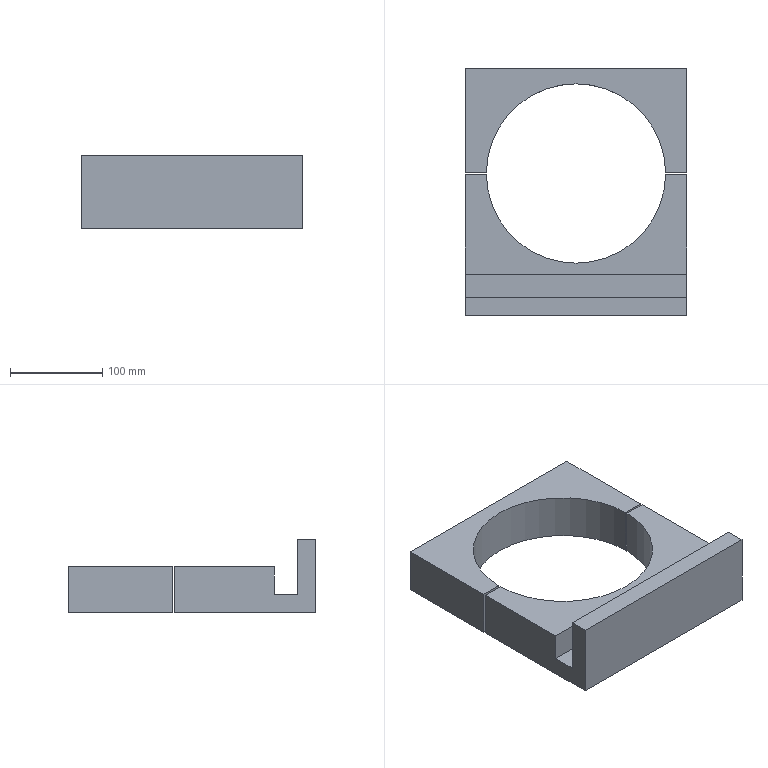Part | STEP file | beam expander fixing.step.STEP-247.STEP | 2 solids | 20 faces | box 240 x 268 x 80 mm | volume 1697437 mm3 | plane 18 | cylinder 2 | commonest cylinder face diameters 194 x2
STEP:
#1=CARTESIAN_POINT('',(96.995,78.,50.));
#2=VERTEX_POINT('',#1);
#3=CARTESIAN_POINT('',(96.995,78.,0.));
#4=VERTEX_POINT('',#3);
#5=CARTESIAN_POINT('',(96.995,78.,50.));
#6=DIRECTION('',(0.,0.,-1.));
#7=VECTOR('',#6,1000.);
#8=LINE('',#5,#7);
#9=EDGE_CURVE('',#2,#4,#8,.T.);
#10=ORIENTED_EDGE('',*,*,#9,.T.);
#11=CARTESIAN_POINT('',(120.,78.,0.));
#12=VERTEX_POINT('',#11);
#13=CARTESIAN_POINT('',(0.,78.,0.));
#14=DIRECTION('',(-1.,0.,0.));
#15=VECTOR('',#14,1000.);
#16=LINE('',#13,#15);
#17=EDGE_CURVE('',#12,#4,#16,.T.);
#18=ORIENTED_EDGE('',*,*,#17,.F.);
#19=CARTESIAN_POINT('',(120.,78.,50.));
#20=VERTEX_POINT('',#19);
#21=CARTESIAN_POINT('',(120.,78.,50.));
#22=DIRECTION('',(0.,0.,1.));
#23=VECTOR('',#22,1000.);
#24=LINE('',#21,#23);
#25=EDGE_CURVE('',#12,#20,#24,.T.);
#26=ORIENTED_EDGE('',*,*,#25,.T.);
#27=CARTESIAN_POINT('',(-163.686,78.,50.));
#28=DIRECTION('',(-1.,0.,0.));
#29=VECTOR('',#28,1000.);
#30=LINE('',#27,#29);
#31=EDGE_CURVE('',#20,#2,#30,.T.);
#32=ORIENTED_EDGE('',*,*,#31,.T.);
#33=EDGE_LOOP('',(#10,#18,#26,#32));
#34=FACE_OUTER_BOUND('',#33,.T.);
#35=CARTESIAN_POINT('',(-163.686,78.,0.));
#36=DIRECTION('',(0.,1.,0.));
#37=DIRECTION('',(1.,0.,0.));
#38=AXIS2_PLACEMENT_3D('',#35,#36,#37);
#39=PLANE('',#38);
#40=ADVANCED_FACE('',(#34),#39,.F.);
#41=CARTESIAN_POINT('',(-96.995,78.,0.));
#42=VERTEX_POINT('',#41);
#43=CARTESIAN_POINT('',(-96.995,78.,50.));
#44=VERTEX_POINT('',#43);
#45=CARTESIAN_POINT('',(-96.995,78.,50.));
#46=DIRECTION('',(0.,0.,1.));
#47=VECTOR('',#46,1000.);
#48=LINE('',#45,#47);
#49=EDGE_CURVE('',#42,#44,#48,.T.);
#50=ORIENTED_EDGE('',*,*,#49,.T.);
#51=CARTESIAN_POINT('',(-120.,78.,50.));
#52=VERTEX_POINT('',#51);
#53=CARTESIAN_POINT('',(-163.686,78.,50.));
#54=DIRECTION('',(-1.,0.,0.));
#55=VECTOR('',#54,1000.);
#56=LINE('',#53,#55);
#57=EDGE_CURVE('',#44,#52,#56,.T.);
#58=ORIENTED_EDGE('',*,*,#57,.T.);
#59=CARTESIAN_POINT('',(-120.,78.,0.));
#60=VERTEX_POINT('',#59);
#61=CARTESIAN_POINT('',(-120.,78.,50.));
#62=DIRECTION('',(0.,0.,1.));
#63=VECTOR('',#62,1000.);
#64=LINE('',#61,#63);
#65=EDGE_CURVE('',#60,#52,#64,.T.);
#66=ORIENTED_EDGE('',*,*,#65,.F.);
#67=CARTESIAN_POINT('',(0.,78.,0.));
#68=DIRECTION('',(-1.,0.,0.));
#69=VECTOR('',#68,1000.);
#70=LINE('',#67,#69);
#71=EDGE_CURVE('',#42,#60,#70,.T.);
#72=ORIENTED_EDGE('',*,*,#71,.F.);
#73=EDGE_LOOP('',(#50,#58,#66,#72));
#74=FACE_OUTER_BOUND('',#73,.T.);
#75=CARTESIAN_POINT('',(-163.686,78.,0.));
#76=DIRECTION('',(0.,1.,0.));
#77=DIRECTION('',(1.,0.,0.));
#78=AXIS2_PLACEMENT_3D('',#75,#76,#77);
#79=PLANE('',#78);
#80=ADVANCED_FACE('',(#74),#79,.F.);
#81=ORIENTED_EDGE('',*,*,#9,.F.);
#82=CARTESIAN_POINT('',(0.,77.,50.));
#83=DIRECTION('',(0.,0.,1.));
#84=DIRECTION('',(1.,0.,0.));
#85=AXIS2_PLACEMENT_3D('',#82,#83,#84);
#86=CIRCLE('',#85,97.);
#87=EDGE_CURVE('',#2,#44,#86,.T.);
#88=ORIENTED_EDGE('',*,*,#87,.T.);
#89=ORIENTED_EDGE('',*,*,#49,.F.);
#90=CARTESIAN_POINT('',(0.,77.,0.));
#91=DIRECTION('',(0.,0.,1.));
#92=DIRECTION('',(1.,0.,0.));
#93=AXIS2_PLACEMENT_3D('',#90,#91,#92);
#94=CIRCLE('',#93,97.);
#95=EDGE_CURVE('',#4,#42,#94,.T.);
#96=ORIENTED_EDGE('',*,*,#95,.F.);
#97=EDGE_LOOP('',(#81,#88,#89,#96));
#98=FACE_OUTER_BOUND('',#97,.T.);
#99=CARTESIAN_POINT('',(0.,77.,50.));
#100=DIRECTION('',(0.,0.,-1.));
#101=DIRECTION('',(-1.,0.,0.));
#102=AXIS2_PLACEMENT_3D('',#99,#100,#101);
#103=CYLINDRICAL_SURFACE('',#102,97.);
#104=ADVANCED_FACE('',(#98),#103,.F.);
#105=CARTESIAN_POINT('',(-120.,191.,0.));
#106=VERTEX_POINT('',#105);
#107=CARTESIAN_POINT('',(-120.,0.,0.));
#108=DIRECTION('',(0.,-1.,0.));
#109=VECTOR('',#108,1000.);
#110=LINE('',#107,#109);
#111=EDGE_CURVE('',#106,#60,#110,.T.);
#112=ORIENTED_EDGE('',*,*,#111,.T.);
#113=ORIENTED_EDGE('',*,*,#65,.T.);
#114=CARTESIAN_POINT('',(-120.,191.,50.));
#115=VERTEX_POINT('',#114);
#116=CARTESIAN_POINT('',(-120.,0.,50.));
#117=DIRECTION('',(0.,-1.,0.));
#118=VECTOR('',#117,1000.);
#119=LINE('',#116,#118);
#120=EDGE_CURVE('',#115,#52,#119,.T.);
#121=ORIENTED_EDGE('',*,*,#120,.F.);
#122=CARTESIAN_POINT('',(-120.,191.,0.));
#123=DIRECTION('',(0.,0.,1.));
#124=VECTOR('',#123,1000.);
#125=LINE('',#122,#124);
#126=EDGE_CURVE('',#106,#115,#125,.T.);
#127=ORIENTED_EDGE('',*,*,#126,.F.);
#128=EDGE_LOOP('',(#112,#113,#121,#127));
#129=FACE_OUTER_BOUND('',#128,.T.);
#130=CARTESIAN_POINT('',(-120.,0.,50.));
#131=DIRECTION('',(1.,0.,0.));
#132=DIRECTION('',(0.,1.,0.));
#133=AXIS2_PLACEMENT_3D('',#130,#131,#132);
#134=PLANE('',#133);
#135=ADVANCED_FACE('',(#129),#134,.F.);
#136=ORIENTED_EDGE('',*,*,#25,.F.);
#137=CARTESIAN_POINT('',(120.,191.,0.));
#138=VERTEX_POINT('',#137);
#139=CARTESIAN_POINT('',(120.,0.,0.));
#140=DIRECTION('',(0.,-1.,0.));
#141=VECTOR('',#140,1000.);
#142=LINE('',#139,#141);
#143=EDGE_CURVE('',#138,#12,#142,.T.);
#144=ORIENTED_EDGE('',*,*,#143,.F.);
#145=CARTESIAN_POINT('',(120.,191.,50.));
#146=VERTEX_POINT('',#145);
#147=CARTESIAN_POINT('',(120.,191.,0.));
#148=DIRECTION('',(0.,0.,1.));
#149=VECTOR('',#148,1000.);
#150=LINE('',#147,#149);
#151=EDGE_CURVE('',#138,#146,#150,.T.);
#152=ORIENTED_EDGE('',*,*,#151,.T.);
#153=CARTESIAN_POINT('',(120.,0.,50.));
#154=DIRECTION('',(0.,-1.,0.));
#155=VECTOR('',#154,1000.);
#156=LINE('',#153,#155);
#157=EDGE_CURVE('',#146,#20,#156,.T.);
#158=ORIENTED_EDGE('',*,*,#157,.T.);
#159=EDGE_LOOP('',(#136,#144,#152,#158));
#160=FACE_OUTER_BOUND('',#159,.T.);
#161=CARTESIAN_POINT('',(120.,0.,50.));
#162=DIRECTION('',(1.,0.,0.));
#163=DIRECTION('',(0.,1.,0.));
#164=AXIS2_PLACEMENT_3D('',#161,#162,#163);
#165=PLANE('',#164);
#166=ADVANCED_FACE('',(#160),#165,.T.);
#167=ORIENTED_EDGE('',*,*,#143,.T.);
#168=ORIENTED_EDGE('',*,*,#17,.T.);
#169=ORIENTED_EDGE('',*,*,#95,.T.);
#170=ORIENTED_EDGE('',*,*,#71,.T.);
#171=ORIENTED_EDGE('',*,*,#111,.F.);
#172=CARTESIAN_POINT('',(-120.,191.,0.));
#173=DIRECTION('',(1.,0.,0.));
#174=VECTOR('',#173,1000.);
#175=LINE('',#172,#174);
#176=EDGE_CURVE('',#106,#138,#175,.T.);
#177=ORIENTED_EDGE('',*,*,#176,.T.);
#178=EDGE_LOOP('',(#167,#168,#169,#170,#171,#177));
#179=FACE_OUTER_BOUND('',#178,.T.);
#180=CARTESIAN_POINT('',(0.,0.,0.));
#181=DIRECTION('',(0.,0.,1.));
#182=DIRECTION('',(1.,0.,0.));
#183=AXIS2_PLACEMENT_3D('',#180,#181,#182);
#184=PLANE('',#183);
#185=ADVANCED_FACE('',(#179),#184,.F.);
#186=ORIENTED_EDGE('',*,*,#31,.F.);
#187=ORIENTED_EDGE('',*,*,#157,.F.);
#188=CARTESIAN_POINT('',(-120.,191.,50.));
#189=DIRECTION('',(1.,0.,0.));
#190=VECTOR('',#189,1000.);
#191=LINE('',#188,#190);
#192=EDGE_CURVE('',#115,#146,#191,.T.);
#193=ORIENTED_EDGE('',*,*,#192,.F.);
#194=ORIENTED_EDGE('',*,*,#120,.T.);
#195=ORIENTED_EDGE('',*,*,#57,.F.);
#196=ORIENTED_EDGE('',*,*,#87,.F.);
#197=EDGE_LOOP('',(#186,#187,#193,#194,#195,#196));
#198=FACE_OUTER_BOUND('',#197,.T.);
#199=CARTESIAN_POINT('',(0.,0.,50.));
#200=DIRECTION('',(0.,0.,1.));
#201=DIRECTION('',(1.,0.,0.));
#202=AXIS2_PLACEMENT_3D('',#199,#200,#201);
#203=PLANE('',#202);
#204=ADVANCED_FACE('',(#198),#203,.T.);
#205=ORIENTED_EDGE('',*,*,#192,.T.);
#206=ORIENTED_EDGE('',*,*,#151,.F.);
#207=ORIENTED_EDGE('',*,*,#176,.F.);
#208=ORIENTED_EDGE('',*,*,#126,.T.);
#209=EDGE_LOOP('',(#205,#206,#207,#208));
#210=FACE_OUTER_BOUND('',#209,.T.);
#211=CARTESIAN_POINT('',(-120.,191.,0.));
#212=DIRECTION('',(0.,-1.,0.));
#213=DIRECTION('',(0.,0.,-1.));
#214=AXIS2_PLACEMENT_3D('',#211,#212,#213);
#215=PLANE('',#214);
#216=ADVANCED_FACE('',(#210),#215,.F.);
#217=CLOSED_SHELL('',(#40,#80,#104,#135,#166,#185,#204,#216));
#218=MANIFOLD_SOLID_BREP('',#217);
#219=CARTESIAN_POINT('',(120.,-57.,20.));
#220=VERTEX_POINT('',#219);
#221=CARTESIAN_POINT('',(120.,-32.,20.));
#222=VERTEX_POINT('',#221);
#223=CARTESIAN_POINT('',(120.,-57.,20.));
#224=DIRECTION('',(0.,1.,0.));
#225=VECTOR('',#224,1000.);
#226=LINE('',#223,#225);
#227=EDGE_CURVE('',#220,#222,#226,.T.);
#228=ORIENTED_EDGE('',*,*,#227,.T.);
#229=CARTESIAN_POINT('',(-120.,-32.,20.));
#230=VERTEX_POINT('',#229);
#231=CARTESIAN_POINT('',(120.,-32.,20.));
#232=DIRECTION('',(-1.,0.,0.));
#233=VECTOR('',#232,1000.);
#234=LINE('',#231,#233);
#235=EDGE_CURVE('',#222,#230,#234,.T.);
#236=ORIENTED_EDGE('',*,*,#235,.T.);
#237=CARTESIAN_POINT('',(-120.,-57.,20.));
#238=VERTEX_POINT('',#237);
#239=CARTESIAN_POINT('',(-120.,-57.,20.));
#240=DIRECTION('',(0.,-1.,0.));
#241=VECTOR('',#240,1000.);
#242=LINE('',#239,#241);
#243=EDGE_CURVE('',#230,#238,#242,.T.);
#244=ORIENTED_EDGE('',*,*,#243,.T.);
#245=CARTESIAN_POINT('',(120.,-57.,20.));
#246=DIRECTION('',(1.,0.,0.));
#247=VECTOR('',#246,1000.);
#248=LINE('',#245,#247);
#249=EDGE_CURVE('',#238,#220,#248,.T.);
#250=ORIENTED_EDGE('',*,*,#249,.T.);
#251=EDGE_LOOP('',(#228,#236,#244,#250));
#252=FACE_OUTER_BOUND('',#251,.T.);
#253=CARTESIAN_POINT('',(0.,0.,20.));
#254=DIRECTION('',(0.,0.,1.));
#255=DIRECTION('',(1.,0.,0.));
#256=AXIS2_PLACEMENT_3D('',#253,#254,#255);
#257=PLANE('',#256);
#258=ADVANCED_FACE('',(#252),#257,.T.);
#259=CARTESIAN_POINT('',(120.,-32.,50.));
#260=VERTEX_POINT('',#259);
#261=CARTESIAN_POINT('',(-120.,-32.,50.));
#262=VERTEX_POINT('',#261);
#263=CARTESIAN_POINT('',(120.,-32.,50.));
#264=DIRECTION('',(-1.,0.,0.));
#265=VECTOR('',#264,1000.);
#266=LINE('',#263,#265);
#267=EDGE_CURVE('',#260,#262,#266,.T.);
#268=ORIENTED_EDGE('',*,*,#267,.T.);
#269=CARTESIAN_POINT('',(-120.,-32.,20.));
#270=DIRECTION('',(0.,0.,1.));
#271=VECTOR('',#270,1000.);
#272=LINE('',#269,#271);
#273=EDGE_CURVE('',#230,#262,#272,.T.);
#274=ORIENTED_EDGE('',*,*,#273,.F.);
#275=ORIENTED_EDGE('',*,*,#235,.F.);
#276=CARTESIAN_POINT('',(120.,-32.,20.));
#277=DIRECTION('',(0.,0.,1.));
#278=VECTOR('',#277,1000.);
#279=LINE('',#276,#278);
#280=EDGE_CURVE('',#222,#260,#279,.T.);
#281=ORIENTED_EDGE('',*,*,#280,.T.);
#282=EDGE_LOOP('',(#268,#274,#275,#281));
#283=FACE_OUTER_BOUND('',#282,.T.);
#284=CARTESIAN_POINT('',(120.,-32.,20.));
#285=DIRECTION('',(0.,1.,0.));
#286=DIRECTION('',(1.,0.,0.));
#287=AXIS2_PLACEMENT_3D('',#284,#285,#286);
#288=PLANE('',#287);
#289=ADVANCED_FACE('',(#283),#288,.F.);
#290=CARTESIAN_POINT('',(-120.,-57.,80.));
#291=VERTEX_POINT('',#290);
#292=CARTESIAN_POINT('',(-120.,-77.,80.));
#293=VERTEX_POINT('',#292);
#294=CARTESIAN_POINT('',(-120.,-77.,80.));
#295=DIRECTION('',(0.,-1.,0.));
#296=VECTOR('',#295,1000.);
#297=LINE('',#294,#296);
#298=EDGE_CURVE('',#291,#293,#297,.T.);
#299=ORIENTED_EDGE('',*,*,#298,.T.);
#300=CARTESIAN_POINT('',(120.,-77.,80.));
#301=VERTEX_POINT('',#300);
#302=CARTESIAN_POINT('',(-120.,-77.,80.));
#303=DIRECTION('',(1.,0.,0.));
#304=VECTOR('',#303,1000.);
#305=LINE('',#302,#304);
#306=EDGE_CURVE('',#293,#301,#305,.T.);
#307=ORIENTED_EDGE('',*,*,#306,.T.);
#308=CARTESIAN_POINT('',(120.,-57.,80.));
#309=VERTEX_POINT('',#308);
#310=CARTESIAN_POINT('',(120.,-77.,80.));
#311=DIRECTION('',(0.,1.,0.));
#312=VECTOR('',#311,1000.);
#313=LINE('',#310,#312);
#314=EDGE_CURVE('',#301,#309,#313,.T.);
#315=ORIENTED_EDGE('',*,*,#314,.T.);
#316=CARTESIAN_POINT('',(-120.,-57.,80.));
#317=DIRECTION('',(-1.,0.,0.));
#318=VECTOR('',#317,1000.);
#319=LINE('',#316,#318);
#320=EDGE_CURVE('',#309,#291,#319,.T.);
#321=ORIENTED_EDGE('',*,*,#320,.T.);
#322=EDGE_LOOP('',(#299,#307,#315,#321));
#323=FACE_OUTER_BOUND('',#322,.T.);
#324=CARTESIAN_POINT('',(0.,0.,80.));
#325=DIRECTION('',(0.,0.,-1.));
#326=DIRECTION('',(0.,-1.,0.));
#327=AXIS2_PLACEMENT_3D('',#324,#325,#326);
#328=PLANE('',#327);
#329=ADVANCED_FACE('',(#323),#328,.F.);
#330=CARTESIAN_POINT('',(120.,-57.,80.));
#331=DIRECTION('',(0.,0.,-1.));
#332=VECTOR('',#331,1000.);
#333=LINE('',#330,#332);
#334=EDGE_CURVE('',#309,#220,#333,.T.);
#335=ORIENTED_EDGE('',*,*,#334,.T.);
#336=ORIENTED_EDGE('',*,*,#249,.F.);
#337=CARTESIAN_POINT('',(-120.,-57.,80.));
#338=DIRECTION('',(0.,0.,-1.));
#339=VECTOR('',#338,1000.);
#340=LINE('',#337,#339);
#341=EDGE_CURVE('',#291,#238,#340,.T.);
#342=ORIENTED_EDGE('',*,*,#341,.F.);
#343=ORIENTED_EDGE('',*,*,#320,.F.);
#344=EDGE_LOOP('',(#335,#336,#342,#343));
#345=FACE_OUTER_BOUND('',#344,.T.);
#346=CARTESIAN_POINT('',(-120.,-57.,80.));
#347=DIRECTION('',(0.,-1.,0.));
#348=DIRECTION('',(0.,0.,-1.));
#349=AXIS2_PLACEMENT_3D('',#346,#347,#348);
#350=PLANE('',#349);
#351=ADVANCED_FACE('',(#345),#350,.F.);
#352=CARTESIAN_POINT('',(-96.995,76.,50.));
#353=VERTEX_POINT('',#352);
#354=CARTESIAN_POINT('',(-96.995,76.,0.));
#355=VERTEX_POINT('',#354);
#356=CARTESIAN_POINT('',(-96.995,76.,50.));
#357=DIRECTION('',(0.,0.,-1.));
#358=VECTOR('',#357,1000.);
#359=LINE('',#356,#358);
#360=EDGE_CURVE('',#353,#355,#359,.T.);
#361=ORIENTED_EDGE('',*,*,#360,.T.);
#362=CARTESIAN_POINT('',(-120.,76.,0.));
#363=VERTEX_POINT('',#362);
#364=CARTESIAN_POINT('',(0.,76.,0.));
#365=DIRECTION('',(1.,0.,0.));
#366=VECTOR('',#365,1000.);
#367=LINE('',#364,#366);
#368=EDGE_CURVE('',#363,#355,#367,.T.);
#369=ORIENTED_EDGE('',*,*,#368,.F.);
#370=CARTESIAN_POINT('',(-120.,76.,50.));
#371=VERTEX_POINT('',#370);
#372=CARTESIAN_POINT('',(-120.,76.,50.));
#373=DIRECTION('',(0.,0.,-1.));
#374=VECTOR('',#373,1000.);
#375=LINE('',#372,#374);
#376=EDGE_CURVE('',#371,#363,#375,.T.);
#377=ORIENTED_EDGE('',*,*,#376,.F.);
#378=CARTESIAN_POINT('',(-163.686,76.,50.));
#379=DIRECTION('',(1.,0.,0.));
#380=VECTOR('',#379,1000.);
#381=LINE('',#378,#380);
#382=EDGE_CURVE('',#371,#353,#381,.T.);
#383=ORIENTED_EDGE('',*,*,#382,.T.);
#384=EDGE_LOOP('',(#361,#369,#377,#383));
#385=FACE_OUTER_BOUND('',#384,.T.);
#386=CARTESIAN_POINT('',(-163.686,76.,0.));
#387=DIRECTION('',(0.,-1.,0.));
#388=DIRECTION('',(0.,0.,-1.));
#389=AXIS2_PLACEMENT_3D('',#386,#387,#388);
#390=PLANE('',#389);
#391=ADVANCED_FACE('',(#385),#390,.F.);
#392=CARTESIAN_POINT('',(96.995,76.,0.));
#393=VERTEX_POINT('',#392);
#394=CARTESIAN_POINT('',(96.995,76.,50.));
#395=VERTEX_POINT('',#394);
#396=CARTESIAN_POINT('',(96.995,76.,50.));
#397=DIRECTION('',(0.,0.,1.));
#398=VECTOR('',#397,1000.);
#399=LINE('',#396,#398);
#400=EDGE_CURVE('',#393,#395,#399,.T.);
#401=ORIENTED_EDGE('',*,*,#400,.T.);
#402=CARTESIAN_POINT('',(120.,76.,50.));
#403=VERTEX_POINT('',#402);
#404=CARTESIAN_POINT('',(-163.686,76.,50.));
#405=DIRECTION('',(1.,0.,0.));
#406=VECTOR('',#405,1000.);
#407=LINE('',#404,#406);
#408=EDGE_CURVE('',#395,#403,#407,.T.);
#409=ORIENTED_EDGE('',*,*,#408,.T.);
#410=CARTESIAN_POINT('',(120.,76.,0.));
#411=VERTEX_POINT('',#410);
#412=CARTESIAN_POINT('',(120.,76.,50.));
#413=DIRECTION('',(0.,0.,-1.));
#414=VECTOR('',#413,1000.);
#415=LINE('',#412,#414);
#416=EDGE_CURVE('',#403,#411,#415,.T.);
#417=ORIENTED_EDGE('',*,*,#416,.T.);
#418=CARTESIAN_POINT('',(0.,76.,0.));
#419=DIRECTION('',(1.,0.,0.));
#420=VECTOR('',#419,1000.);
#421=LINE('',#418,#420);
#422=EDGE_CURVE('',#393,#411,#421,.T.);
#423=ORIENTED_EDGE('',*,*,#422,.F.);
#424=EDGE_LOOP('',(#401,#409,#417,#423));
#425=FACE_OUTER_BOUND('',#424,.T.);
#426=CARTESIAN_POINT('',(-163.686,76.,0.));
#427=DIRECTION('',(0.,-1.,0.));
#428=DIRECTION('',(0.,0.,-1.));
#429=AXIS2_PLACEMENT_3D('',#426,#427,#428);
#430=PLANE('',#429);
#431=ADVANCED_FACE('',(#425),#430,.F.);
#432=CARTESIAN_POINT('',(-120.,-77.,0.));
#433=VERTEX_POINT('',#432);
#434=CARTESIAN_POINT('',(120.,-77.,0.));
#435=VERTEX_POINT('',#434);
#436=CARTESIAN_POINT('',(0.,-77.,0.));
#437=DIRECTION('',(1.,0.,0.));
#438=VECTOR('',#437,1000.);
#439=LINE('',#436,#438);
#440=EDGE_CURVE('',#433,#435,#439,.T.);
#441=ORIENTED_EDGE('',*,*,#440,.T.);
#442=CARTESIAN_POINT('',(120.,-77.,50.));
#443=DIRECTION('',(0.,0.,-1.));
#444=VECTOR('',#443,1000.);
#445=LINE('',#442,#444);
#446=EDGE_CURVE('',#301,#435,#445,.T.);
#447=ORIENTED_EDGE('',*,*,#446,.F.);
#448=ORIENTED_EDGE('',*,*,#306,.F.);
#449=CARTESIAN_POINT('',(-120.,-77.,50.));
#450=DIRECTION('',(0.,0.,-1.));
#451=VECTOR('',#450,1000.);
#452=LINE('',#449,#451);
#453=EDGE_CURVE('',#293,#433,#452,.T.);
#454=ORIENTED_EDGE('',*,*,#453,.T.);
#455=EDGE_LOOP('',(#441,#447,#448,#454));
#456=FACE_OUTER_BOUND('',#455,.T.);
#457=CARTESIAN_POINT('',(0.,-77.,50.));
#458=DIRECTION('',(0.,1.,0.));
#459=DIRECTION('',(1.,0.,0.));
#460=AXIS2_PLACEMENT_3D('',#457,#458,#459);
#461=PLANE('',#460);
#462=ADVANCED_FACE('',(#456),#461,.F.);
#463=CARTESIAN_POINT('',(-120.,0.,0.));
#464=DIRECTION('',(0.,-1.,0.));
#465=VECTOR('',#464,1000.);
#466=LINE('',#463,#465);
#467=EDGE_CURVE('',#363,#433,#466,.T.);
#468=ORIENTED_EDGE('',*,*,#467,.F.);
#469=ORIENTED_EDGE('',*,*,#368,.T.);
#470=CARTESIAN_POINT('',(0.,77.,0.));
#471=DIRECTION('',(0.,0.,1.));
#472=DIRECTION('',(1.,0.,0.));
#473=AXIS2_PLACEMENT_3D('',#470,#471,#472);
#474=CIRCLE('',#473,97.);
#475=EDGE_CURVE('',#355,#393,#474,.T.);
#476=ORIENTED_EDGE('',*,*,#475,.T.);
#477=ORIENTED_EDGE('',*,*,#422,.T.);
#478=CARTESIAN_POINT('',(120.,0.,0.));
#479=DIRECTION('',(0.,-1.,0.));
#480=VECTOR('',#479,1000.);
#481=LINE('',#478,#480);
#482=EDGE_CURVE('',#411,#435,#481,.T.);
#483=ORIENTED_EDGE('',*,*,#482,.T.);
#484=ORIENTED_EDGE('',*,*,#440,.F.);
#485=EDGE_LOOP('',(#468,#469,#476,#477,#483,#484));
#486=FACE_OUTER_BOUND('',#485,.T.);
#487=CARTESIAN_POINT('',(0.,0.,0.));
#488=DIRECTION('',(0.,0.,1.));
#489=DIRECTION('',(1.,0.,0.));
#490=AXIS2_PLACEMENT_3D('',#487,#488,#489);
#491=PLANE('',#490);
#492=ADVANCED_FACE('',(#486),#491,.F.);
#493=ORIENTED_EDGE('',*,*,#267,.F.);
#494=CARTESIAN_POINT('',(120.,0.,50.));
#495=DIRECTION('',(0.,-1.,0.));
#496=VECTOR('',#495,1000.);
#497=LINE('',#494,#496);
#498=EDGE_CURVE('',#403,#260,#497,.T.);
#499=ORIENTED_EDGE('',*,*,#498,.F.);
#500=ORIENTED_EDGE('',*,*,#408,.F.);
#501=CARTESIAN_POINT('',(0.,77.,50.));
#502=DIRECTION('',(0.,0.,1.));
#503=DIRECTION('',(1.,0.,0.));
#504=AXIS2_PLACEMENT_3D('',#501,#502,#503);
#505=CIRCLE('',#504,97.);
#506=EDGE_CURVE('',#353,#395,#505,.T.);
#507=ORIENTED_EDGE('',*,*,#506,.F.);
#508=ORIENTED_EDGE('',*,*,#382,.F.);
#509=CARTESIAN_POINT('',(-120.,0.,50.));
#510=DIRECTION('',(0.,-1.,0.));
#511=VECTOR('',#510,1000.);
#512=LINE('',#509,#511);
#513=EDGE_CURVE('',#371,#262,#512,.T.);
#514=ORIENTED_EDGE('',*,*,#513,.T.);
#515=EDGE_LOOP('',(#493,#499,#500,#507,#508,#514));
#516=FACE_OUTER_BOUND('',#515,.T.);
#517=CARTESIAN_POINT('',(0.,0.,50.));
#518=DIRECTION('',(0.,0.,1.));
#519=DIRECTION('',(1.,0.,0.));
#520=AXIS2_PLACEMENT_3D('',#517,#518,#519);
#521=PLANE('',#520);
#522=ADVANCED_FACE('',(#516),#521,.T.);
#523=ORIENTED_EDGE('',*,*,#227,.F.);
#524=ORIENTED_EDGE('',*,*,#334,.F.);
#525=ORIENTED_EDGE('',*,*,#314,.F.);
#526=ORIENTED_EDGE('',*,*,#446,.T.);
#527=ORIENTED_EDGE('',*,*,#482,.F.);
#528=ORIENTED_EDGE('',*,*,#416,.F.);
#529=ORIENTED_EDGE('',*,*,#498,.T.);
#530=ORIENTED_EDGE('',*,*,#280,.F.);
#531=EDGE_LOOP('',(#523,#524,#525,#526,#527,#528,#529,#530));
#532=FACE_OUTER_BOUND('',#531,.T.);
#533=CARTESIAN_POINT('',(120.,0.,50.));
#534=DIRECTION('',(1.,0.,0.));
#535=DIRECTION('',(0.,1.,0.));
#536=AXIS2_PLACEMENT_3D('',#533,#534,#535);
#537=PLANE('',#536);
#538=ADVANCED_FACE('',(#532),#537,.T.);
#539=ORIENTED_EDGE('',*,*,#341,.T.);
#540=ORIENTED_EDGE('',*,*,#243,.F.);
#541=ORIENTED_EDGE('',*,*,#273,.T.);
#542=ORIENTED_EDGE('',*,*,#513,.F.);
#543=ORIENTED_EDGE('',*,*,#376,.T.);
#544=ORIENTED_EDGE('',*,*,#467,.T.);
#545=ORIENTED_EDGE('',*,*,#453,.F.);
#546=ORIENTED_EDGE('',*,*,#298,.F.);
#547=EDGE_LOOP('',(#539,#540,#541,#542,#543,#544,#545,#546));
#548=FACE_OUTER_BOUND('',#547,.T.);
#549=CARTESIAN_POINT('',(-120.,0.,50.));
#550=DIRECTION('',(1.,0.,0.));
#551=DIRECTION('',(0.,1.,0.));
#552=AXIS2_PLACEMENT_3D('',#549,#550,#551);
#553=PLANE('',#552);
#554=ADVANCED_FACE('',(#548),#553,.F.);
#555=ORIENTED_EDGE('',*,*,#360,.F.);
#556=ORIENTED_EDGE('',*,*,#506,.T.);
#557=ORIENTED_EDGE('',*,*,#400,.F.);
#558=ORIENTED_EDGE('',*,*,#475,.F.);
#559=EDGE_LOOP('',(#555,#556,#557,#558));
#560=FACE_OUTER_BOUND('',#559,.T.);
#561=CARTESIAN_POINT('',(0.,77.,50.));
#562=DIRECTION('',(0.,0.,-1.));
#563=DIRECTION('',(-1.,0.,0.));
#564=AXIS2_PLACEMENT_3D('',#561,#562,#563);
#565=CYLINDRICAL_SURFACE('',#564,97.);
#566=ADVANCED_FACE('',(#560),#565,.F.);
#567=CLOSED_SHELL('',(#258,#289,#329,#351,#391,#431,#462,#492,#522,#538,#554,#566));
#568=MANIFOLD_SOLID_BREP('',#567);
#569=CARTESIAN_POINT('',(0.,0.,0.));
#570=DIRECTION('',(0.,0.,1.));
#571=DIRECTION('',(1.,0.,0.));
#572=AXIS2_PLACEMENT_3D('',#569,#570,#571);
#573=(LENGTH_UNIT()NAMED_UNIT(*)SI_UNIT(.MILLI.,.METRE.));
#574=UNCERTAINTY_MEASURE_WITH_UNIT(LENGTH_MEASURE(0.00001),#573,'','');
#575=(NAMED_UNIT(*)PLANE_ANGLE_UNIT()SI_UNIT($,.RADIAN.));
#576=(NAMED_UNIT(*)SI_UNIT($,.STERADIAN.)SOLID_ANGLE_UNIT());
#577=(GEOMETRIC_REPRESENTATION_CONTEXT(3)GLOBAL_UNCERTAINTY_ASSIGNED_CONTEXT((#574))GLOBAL_UNIT_ASSIGNED_CONTEXT((#573,#575,#576))REPRESENTATION_CONTEXT('',''));
#578=ADVANCED_BREP_SHAPE_REPRESENTATION('',(#218,#568,#572),#577);